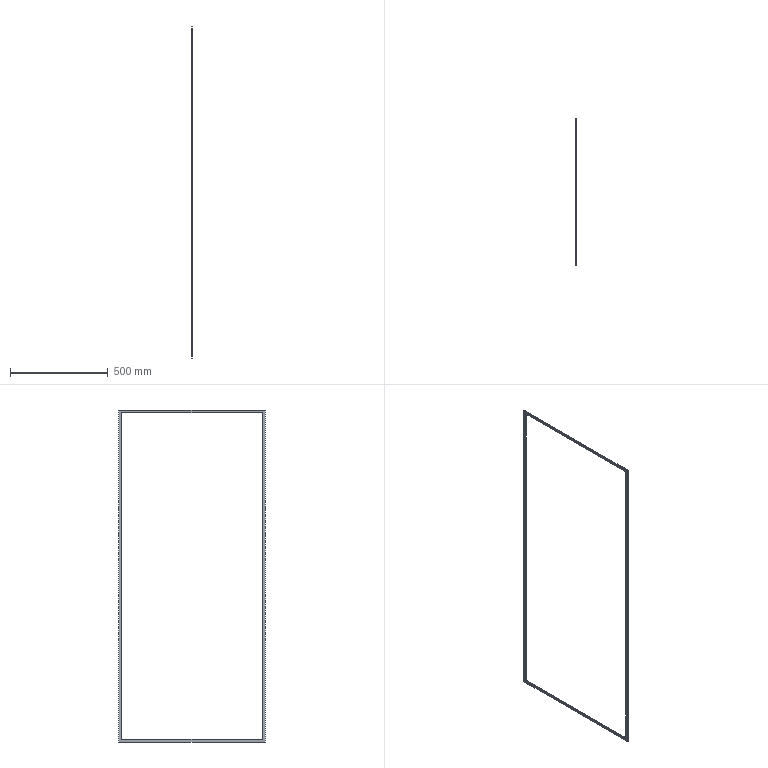Part | STEP file | RJWD-DY-0102_X2_5DE667DC95E8_44 | 1 solid | 10 faces | box 3 x 752 x 1702 mm | volume 218115 mm3 | plane 10
STEP:
#1=CARTESIAN_POINT('',(0.,0.,0.));
#2=DIRECTION('',(0.,0.,1.));
#3=DIRECTION('',(1.,0.,0.));
#4=AXIS2_PLACEMENT_3D('',#1,#2,#3);
#5=CARTESIAN_POINT('',(-521.773,4998.173,1734.894));
#6=VERTEX_POINT('',#5);
#7=CARTESIAN_POINT('',(-521.773,4246.173,1734.894));
#8=VERTEX_POINT('',#7);
#9=CARTESIAN_POINT('',(-521.773,4998.173,1734.894));
#10=DIRECTION('',(0.,-1.,0.));
#11=VECTOR('',#10,1.);
#12=LINE('',#9,#11);
#13=CARTESIAN_POINT('',(-521.773,4622.173,884.144));
#14=DIRECTION('',(-1.,0.,0.));
#15=DIRECTION('',(0.,0.,1.));
#16=AXIS2_PLACEMENT_3D('',#13,#14,#15);
#17=PLANE('',#16);
#18=CARTESIAN_POINT('',(850.75,376.));
#19=DIRECTION('',(0.,-1.));
#20=VECTOR('',#19,1.);
#21=LINE('',#18,#20);
#22=(GEOMETRIC_REPRESENTATION_CONTEXT(2)PARAMETRIC_REPRESENTATION_CONTEXT()REPRESENTATION_CONTEXT('',''));
#23=DEFINITIONAL_REPRESENTATION('',(#21),#22);
#24=PCURVE('',#17,#23);
#25=CARTESIAN_POINT('',(-521.773,4246.173,1734.894));
#26=DIRECTION('',(0.,0.,1.));
#27=DIRECTION('',(0.,-1.,0.));
#28=AXIS2_PLACEMENT_3D('',#25,#26,#27);
#29=PLANE('',#28);
#30=CARTESIAN_POINT('',(-752.,0.));
#31=DIRECTION('',(1.,0.));
#32=VECTOR('',#31,1.);
#33=LINE('',#30,#32);
#34=(GEOMETRIC_REPRESENTATION_CONTEXT(2)PARAMETRIC_REPRESENTATION_CONTEXT()REPRESENTATION_CONTEXT('',''));
#35=DEFINITIONAL_REPRESENTATION('',(#33),#34);
#36=PCURVE('',#29,#35);
#37=SURFACE_CURVE('',#12,(#24,#36),.PCURVE_S1.);
#38=EDGE_CURVE('',#6,#8,#37,.T.);
#39=ORIENTED_EDGE('',*,*,#38,.F.);
#40=CARTESIAN_POINT('',(-521.773,4998.173,33.394));
#41=VERTEX_POINT('',#40);
#42=CARTESIAN_POINT('',(-521.773,4998.173,33.394));
#43=DIRECTION('',(0.,0.,1.));
#44=VECTOR('',#43,1.);
#45=LINE('',#42,#44);
#46=CARTESIAN_POINT('',(-850.75,376.));
#47=DIRECTION('',(1.,0.));
#48=VECTOR('',#47,1.);
#49=LINE('',#46,#48);
#50=(GEOMETRIC_REPRESENTATION_CONTEXT(2)PARAMETRIC_REPRESENTATION_CONTEXT()REPRESENTATION_CONTEXT('',''));
#51=DEFINITIONAL_REPRESENTATION('',(#49),#50);
#52=PCURVE('',#17,#51);
#53=CARTESIAN_POINT('',(-521.773,4998.173,1734.894));
#54=DIRECTION('',(0.,1.,0.));
#55=DIRECTION('',(0.,0.,1.));
#56=AXIS2_PLACEMENT_3D('',#53,#54,#55);
#57=PLANE('',#56);
#58=CARTESIAN_POINT('',(-1701.5,0.));
#59=DIRECTION('',(1.,0.));
#60=VECTOR('',#59,1.);
#61=LINE('',#58,#60);
#62=(GEOMETRIC_REPRESENTATION_CONTEXT(2)PARAMETRIC_REPRESENTATION_CONTEXT()REPRESENTATION_CONTEXT('',''));
#63=DEFINITIONAL_REPRESENTATION('',(#61),#62);
#64=PCURVE('',#57,#63);
#65=SURFACE_CURVE('',#45,(#52,#64),.PCURVE_S1.);
#66=EDGE_CURVE('',#41,#6,#65,.T.);
#67=ORIENTED_EDGE('',*,*,#66,.F.);
#68=CARTESIAN_POINT('',(-521.773,4246.173,33.394));
#69=VERTEX_POINT('',#68);
#70=CARTESIAN_POINT('',(-521.773,4246.173,33.394));
#71=DIRECTION('',(0.,1.,0.));
#72=VECTOR('',#71,1.);
#73=LINE('',#70,#72);
#74=CARTESIAN_POINT('',(-850.75,-376.));
#75=DIRECTION('',(0.,1.));
#76=VECTOR('',#75,1.);
#77=LINE('',#74,#76);
#78=(GEOMETRIC_REPRESENTATION_CONTEXT(2)PARAMETRIC_REPRESENTATION_CONTEXT()REPRESENTATION_CONTEXT('',''));
#79=DEFINITIONAL_REPRESENTATION('',(#77),#78);
#80=PCURVE('',#17,#79);
#81=CARTESIAN_POINT('',(-521.773,4998.173,33.394));
#82=DIRECTION('',(0.,0.,-1.));
#83=DIRECTION('',(0.,1.,0.));
#84=AXIS2_PLACEMENT_3D('',#81,#82,#83);
#85=PLANE('',#84);
#86=CARTESIAN_POINT('',(-752.,0.));
#87=DIRECTION('',(1.,0.));
#88=VECTOR('',#87,1.);
#89=LINE('',#86,#88);
#90=(GEOMETRIC_REPRESENTATION_CONTEXT(2)PARAMETRIC_REPRESENTATION_CONTEXT()REPRESENTATION_CONTEXT('',''));
#91=DEFINITIONAL_REPRESENTATION('',(#89),#90);
#92=PCURVE('',#85,#91);
#93=SURFACE_CURVE('',#73,(#80,#92),.PCURVE_S1.);
#94=EDGE_CURVE('',#69,#41,#93,.T.);
#95=ORIENTED_EDGE('',*,*,#94,.F.);
#96=CARTESIAN_POINT('',(-521.773,4246.173,1734.894));
#97=DIRECTION('',(0.,0.,-1.));
#98=VECTOR('',#97,1.);
#99=LINE('',#96,#98);
#100=CARTESIAN_POINT('',(850.75,-376.));
#101=DIRECTION('',(-1.,0.));
#102=VECTOR('',#101,1.);
#103=LINE('',#100,#102);
#104=(GEOMETRIC_REPRESENTATION_CONTEXT(2)PARAMETRIC_REPRESENTATION_CONTEXT()REPRESENTATION_CONTEXT('',''));
#105=DEFINITIONAL_REPRESENTATION('',(#103),#104);
#106=PCURVE('',#17,#105);
#107=CARTESIAN_POINT('',(-521.773,4246.173,33.394));
#108=DIRECTION('',(0.,-1.,0.));
#109=DIRECTION('',(0.,0.,-1.));
#110=AXIS2_PLACEMENT_3D('',#107,#108,#109);
#111=PLANE('',#110);
#112=CARTESIAN_POINT('',(-1701.5,0.));
#113=DIRECTION('',(1.,0.));
#114=VECTOR('',#113,1.);
#115=LINE('',#112,#114);
#116=(GEOMETRIC_REPRESENTATION_CONTEXT(2)PARAMETRIC_REPRESENTATION_CONTEXT()REPRESENTATION_CONTEXT('',''));
#117=DEFINITIONAL_REPRESENTATION('',(#115),#116);
#118=PCURVE('',#111,#117);
#119=SURFACE_CURVE('',#99,(#106,#118),.PCURVE_S1.);
#120=EDGE_CURVE('',#8,#69,#119,.T.);
#121=ORIENTED_EDGE('',*,*,#120,.F.);
#122=EDGE_LOOP('',(#39,#67,#95,#121));
#123=FACE_BOUND('',#122,.F.);
#124=CARTESIAN_POINT('',(-521.773,4983.173,48.394));
#125=VERTEX_POINT('',#124);
#126=CARTESIAN_POINT('',(-521.773,4261.173,48.394));
#127=VERTEX_POINT('',#126);
#128=CARTESIAN_POINT('',(-521.773,4983.173,48.394));
#129=DIRECTION('',(0.,-1.,0.));
#130=VECTOR('',#129,1.);
#131=LINE('',#128,#130);
#132=CARTESIAN_POINT('',(-835.75,361.));
#133=DIRECTION('',(0.,-1.));
#134=VECTOR('',#133,1.);
#135=LINE('',#132,#134);
#136=(GEOMETRIC_REPRESENTATION_CONTEXT(2)PARAMETRIC_REPRESENTATION_CONTEXT()REPRESENTATION_CONTEXT('',''));
#137=DEFINITIONAL_REPRESENTATION('',(#135),#136);
#138=PCURVE('',#17,#137);
#139=CARTESIAN_POINT('',(-521.773,4261.173,48.394));
#140=DIRECTION('',(0.,0.,1.));
#141=DIRECTION('',(0.,-1.,0.));
#142=AXIS2_PLACEMENT_3D('',#139,#140,#141);
#143=PLANE('',#142);
#144=CARTESIAN_POINT('',(-722.,0.));
#145=DIRECTION('',(1.,0.));
#146=VECTOR('',#145,1.);
#147=LINE('',#144,#146);
#148=(GEOMETRIC_REPRESENTATION_CONTEXT(2)PARAMETRIC_REPRESENTATION_CONTEXT()REPRESENTATION_CONTEXT('',''));
#149=DEFINITIONAL_REPRESENTATION('',(#147),#148);
#150=PCURVE('',#143,#149);
#151=SURFACE_CURVE('',#131,(#138,#150),.PCURVE_S1.);
#152=EDGE_CURVE('',#125,#127,#151,.T.);
#153=ORIENTED_EDGE('',*,*,#152,.F.);
#154=CARTESIAN_POINT('',(-521.773,4983.173,1719.894));
#155=VERTEX_POINT('',#154);
#156=CARTESIAN_POINT('',(-521.773,4983.173,48.394));
#157=DIRECTION('',(0.,0.,1.));
#158=VECTOR('',#157,1.);
#159=LINE('',#156,#158);
#160=CARTESIAN_POINT('',(-835.75,361.));
#161=DIRECTION('',(1.,0.));
#162=VECTOR('',#161,1.);
#163=LINE('',#160,#162);
#164=(GEOMETRIC_REPRESENTATION_CONTEXT(2)PARAMETRIC_REPRESENTATION_CONTEXT()REPRESENTATION_CONTEXT('',''));
#165=DEFINITIONAL_REPRESENTATION('',(#163),#164);
#166=PCURVE('',#17,#165);
#167=CARTESIAN_POINT('',(-521.773,4983.173,48.394));
#168=DIRECTION('',(0.,-1.,0.));
#169=DIRECTION('',(0.,0.,-1.));
#170=AXIS2_PLACEMENT_3D('',#167,#168,#169);
#171=PLANE('',#170);
#172=CARTESIAN_POINT('',(0.,0.));
#173=DIRECTION('',(-1.,0.));
#174=VECTOR('',#173,1.);
#175=LINE('',#172,#174);
#176=(GEOMETRIC_REPRESENTATION_CONTEXT(2)PARAMETRIC_REPRESENTATION_CONTEXT()REPRESENTATION_CONTEXT('',''));
#177=DEFINITIONAL_REPRESENTATION('',(#175),#176);
#178=PCURVE('',#171,#177);
#179=SURFACE_CURVE('',#159,(#166,#178),.PCURVE_S1.);
#180=EDGE_CURVE('',#125,#155,#179,.T.);
#181=ORIENTED_EDGE('',*,*,#180,.T.);
#182=CARTESIAN_POINT('',(-521.773,4261.173,1719.894));
#183=VERTEX_POINT('',#182);
#184=CARTESIAN_POINT('',(-521.773,4261.173,1719.894));
#185=DIRECTION('',(0.,1.,0.));
#186=VECTOR('',#185,1.);
#187=LINE('',#184,#186);
#188=CARTESIAN_POINT('',(835.75,-361.));
#189=DIRECTION('',(0.,1.));
#190=VECTOR('',#189,1.);
#191=LINE('',#188,#190);
#192=(GEOMETRIC_REPRESENTATION_CONTEXT(2)PARAMETRIC_REPRESENTATION_CONTEXT()REPRESENTATION_CONTEXT('',''));
#193=DEFINITIONAL_REPRESENTATION('',(#191),#192);
#194=PCURVE('',#17,#193);
#195=CARTESIAN_POINT('',(-521.773,4983.173,1719.894));
#196=DIRECTION('',(0.,0.,-1.));
#197=DIRECTION('',(0.,1.,0.));
#198=AXIS2_PLACEMENT_3D('',#195,#196,#197);
#199=PLANE('',#198);
#200=CARTESIAN_POINT('',(-722.,0.));
#201=DIRECTION('',(1.,0.));
#202=VECTOR('',#201,1.);
#203=LINE('',#200,#202);
#204=(GEOMETRIC_REPRESENTATION_CONTEXT(2)PARAMETRIC_REPRESENTATION_CONTEXT()REPRESENTATION_CONTEXT('',''));
#205=DEFINITIONAL_REPRESENTATION('',(#203),#204);
#206=PCURVE('',#199,#205);
#207=SURFACE_CURVE('',#187,(#194,#206),.PCURVE_S1.);
#208=EDGE_CURVE('',#183,#155,#207,.T.);
#209=ORIENTED_EDGE('',*,*,#208,.F.);
#210=CARTESIAN_POINT('',(-521.773,4261.173,48.394));
#211=DIRECTION('',(0.,0.,1.));
#212=VECTOR('',#211,1.);
#213=LINE('',#210,#212);
#214=CARTESIAN_POINT('',(-835.75,-361.));
#215=DIRECTION('',(1.,0.));
#216=VECTOR('',#215,1.);
#217=LINE('',#214,#216);
#218=(GEOMETRIC_REPRESENTATION_CONTEXT(2)PARAMETRIC_REPRESENTATION_CONTEXT()REPRESENTATION_CONTEXT('',''));
#219=DEFINITIONAL_REPRESENTATION('',(#217),#218);
#220=PCURVE('',#17,#219);
#221=CARTESIAN_POINT('',(-521.773,4261.173,1719.894));
#222=DIRECTION('',(0.,1.,0.));
#223=DIRECTION('',(0.,0.,1.));
#224=AXIS2_PLACEMENT_3D('',#221,#222,#223);
#225=PLANE('',#224);
#226=CARTESIAN_POINT('',(-1671.5,0.));
#227=DIRECTION('',(1.,0.));
#228=VECTOR('',#227,1.);
#229=LINE('',#226,#228);
#230=(GEOMETRIC_REPRESENTATION_CONTEXT(2)PARAMETRIC_REPRESENTATION_CONTEXT()REPRESENTATION_CONTEXT('',''));
#231=DEFINITIONAL_REPRESENTATION('',(#229),#230);
#232=PCURVE('',#225,#231);
#233=SURFACE_CURVE('',#213,(#220,#232),.PCURVE_S1.);
#234=EDGE_CURVE('',#127,#183,#233,.T.);
#235=ORIENTED_EDGE('',*,*,#234,.F.);
#236=EDGE_LOOP('',(#153,#181,#209,#235));
#237=FACE_BOUND('',#236,.F.);
#238=ADVANCED_FACE('',(#123,#237),#17,.F.);
#239=ORIENTED_EDGE('',*,*,#38,.T.);
#240=CARTESIAN_POINT('',(-524.773,4246.173,1734.894));
#241=VERTEX_POINT('',#240);
#242=CARTESIAN_POINT('',(-524.773,4246.173,1734.894));
#243=DIRECTION('',(1.,0.,0.));
#244=VECTOR('',#243,1.);
#245=LINE('',#242,#244);
#246=CARTESIAN_POINT('',(0.,-3.));
#247=DIRECTION('',(0.,1.));
#248=VECTOR('',#247,1.);
#249=LINE('',#246,#248);
#250=(GEOMETRIC_REPRESENTATION_CONTEXT(2)PARAMETRIC_REPRESENTATION_CONTEXT()REPRESENTATION_CONTEXT('',''));
#251=DEFINITIONAL_REPRESENTATION('',(#249),#250);
#252=PCURVE('',#29,#251);
#253=CARTESIAN_POINT('',(-1701.5,-3.));
#254=DIRECTION('',(0.,1.));
#255=VECTOR('',#254,1.);
#256=LINE('',#253,#255);
#257=(GEOMETRIC_REPRESENTATION_CONTEXT(2)PARAMETRIC_REPRESENTATION_CONTEXT()REPRESENTATION_CONTEXT('',''));
#258=DEFINITIONAL_REPRESENTATION('',(#256),#257);
#259=PCURVE('',#111,#258);
#260=SURFACE_CURVE('',#245,(#252,#259),.PCURVE_S1.);
#261=EDGE_CURVE('',#241,#8,#260,.T.);
#262=ORIENTED_EDGE('',*,*,#261,.F.);
#263=CARTESIAN_POINT('',(-524.773,4998.173,1734.894));
#264=VERTEX_POINT('',#263);
#265=CARTESIAN_POINT('',(-524.773,4998.173,1734.894));
#266=DIRECTION('',(0.,-1.,0.));
#267=VECTOR('',#266,1.);
#268=LINE('',#265,#267);
#269=CARTESIAN_POINT('',(-752.,-3.));
#270=DIRECTION('',(1.,0.));
#271=VECTOR('',#270,1.);
#272=LINE('',#269,#271);
#273=(GEOMETRIC_REPRESENTATION_CONTEXT(2)PARAMETRIC_REPRESENTATION_CONTEXT()REPRESENTATION_CONTEXT('',''));
#274=DEFINITIONAL_REPRESENTATION('',(#272),#273);
#275=PCURVE('',#29,#274);
#276=CARTESIAN_POINT('',(-524.773,4622.173,884.144));
#277=DIRECTION('',(-1.,0.,0.));
#278=DIRECTION('',(0.,0.,1.));
#279=AXIS2_PLACEMENT_3D('',#276,#277,#278);
#280=PLANE('',#279);
#281=CARTESIAN_POINT('',(850.75,376.));
#282=DIRECTION('',(0.,-1.));
#283=VECTOR('',#282,1.);
#284=LINE('',#281,#283);
#285=(GEOMETRIC_REPRESENTATION_CONTEXT(2)PARAMETRIC_REPRESENTATION_CONTEXT()REPRESENTATION_CONTEXT('',''));
#286=DEFINITIONAL_REPRESENTATION('',(#284),#285);
#287=PCURVE('',#280,#286);
#288=SURFACE_CURVE('',#268,(#275,#287),.PCURVE_S1.);
#289=EDGE_CURVE('',#264,#241,#288,.T.);
#290=ORIENTED_EDGE('',*,*,#289,.F.);
#291=CARTESIAN_POINT('',(-524.773,4998.173,1734.894));
#292=DIRECTION('',(1.,0.,0.));
#293=VECTOR('',#292,1.);
#294=LINE('',#291,#293);
#295=CARTESIAN_POINT('',(-752.,-3.));
#296=DIRECTION('',(0.,1.));
#297=VECTOR('',#296,1.);
#298=LINE('',#295,#297);
#299=(GEOMETRIC_REPRESENTATION_CONTEXT(2)PARAMETRIC_REPRESENTATION_CONTEXT()REPRESENTATION_CONTEXT('',''));
#300=DEFINITIONAL_REPRESENTATION('',(#298),#299);
#301=PCURVE('',#29,#300);
#302=CARTESIAN_POINT('',(0.,-3.));
#303=DIRECTION('',(0.,1.));
#304=VECTOR('',#303,1.);
#305=LINE('',#302,#304);
#306=(GEOMETRIC_REPRESENTATION_CONTEXT(2)PARAMETRIC_REPRESENTATION_CONTEXT()REPRESENTATION_CONTEXT('',''));
#307=DEFINITIONAL_REPRESENTATION('',(#305),#306);
#308=PCURVE('',#57,#307);
#309=SURFACE_CURVE('',#294,(#301,#308),.PCURVE_S1.);
#310=EDGE_CURVE('',#264,#6,#309,.T.);
#311=ORIENTED_EDGE('',*,*,#310,.T.);
#312=EDGE_LOOP('',(#239,#262,#290,#311));
#313=FACE_BOUND('',#312,.F.);
#314=ADVANCED_FACE('',(#313),#29,.T.);
#315=ORIENTED_EDGE('',*,*,#261,.T.);
#316=ORIENTED_EDGE('',*,*,#120,.T.);
#317=CARTESIAN_POINT('',(-524.773,4246.173,33.394));
#318=VERTEX_POINT('',#317);
#319=CARTESIAN_POINT('',(-524.773,4246.173,33.394));
#320=DIRECTION('',(1.,0.,0.));
#321=VECTOR('',#320,1.);
#322=LINE('',#319,#321);
#323=CARTESIAN_POINT('',(0.,-3.));
#324=DIRECTION('',(0.,1.));
#325=VECTOR('',#324,1.);
#326=LINE('',#323,#325);
#327=(GEOMETRIC_REPRESENTATION_CONTEXT(2)PARAMETRIC_REPRESENTATION_CONTEXT()REPRESENTATION_CONTEXT('',''));
#328=DEFINITIONAL_REPRESENTATION('',(#326),#327);
#329=PCURVE('',#111,#328);
#330=CARTESIAN_POINT('',(-752.,-3.));
#331=DIRECTION('',(0.,1.));
#332=VECTOR('',#331,1.);
#333=LINE('',#330,#332);
#334=(GEOMETRIC_REPRESENTATION_CONTEXT(2)PARAMETRIC_REPRESENTATION_CONTEXT()REPRESENTATION_CONTEXT('',''));
#335=DEFINITIONAL_REPRESENTATION('',(#333),#334);
#336=PCURVE('',#85,#335);
#337=SURFACE_CURVE('',#322,(#329,#336),.PCURVE_S1.);
#338=EDGE_CURVE('',#318,#69,#337,.T.);
#339=ORIENTED_EDGE('',*,*,#338,.F.);
#340=CARTESIAN_POINT('',(-524.773,4246.173,1734.894));
#341=DIRECTION('',(0.,0.,-1.));
#342=VECTOR('',#341,1.);
#343=LINE('',#340,#342);
#344=CARTESIAN_POINT('',(-1701.5,-3.));
#345=DIRECTION('',(1.,0.));
#346=VECTOR('',#345,1.);
#347=LINE('',#344,#346);
#348=(GEOMETRIC_REPRESENTATION_CONTEXT(2)PARAMETRIC_REPRESENTATION_CONTEXT()REPRESENTATION_CONTEXT('',''));
#349=DEFINITIONAL_REPRESENTATION('',(#347),#348);
#350=PCURVE('',#111,#349);
#351=CARTESIAN_POINT('',(850.75,-376.));
#352=DIRECTION('',(-1.,0.));
#353=VECTOR('',#352,1.);
#354=LINE('',#351,#353);
#355=(GEOMETRIC_REPRESENTATION_CONTEXT(2)PARAMETRIC_REPRESENTATION_CONTEXT()REPRESENTATION_CONTEXT('',''));
#356=DEFINITIONAL_REPRESENTATION('',(#354),#355);
#357=PCURVE('',#280,#356);
#358=SURFACE_CURVE('',#343,(#350,#357),.PCURVE_S1.);
#359=EDGE_CURVE('',#241,#318,#358,.T.);
#360=ORIENTED_EDGE('',*,*,#359,.F.);
#361=EDGE_LOOP('',(#315,#316,#339,#360));
#362=FACE_BOUND('',#361,.F.);
#363=ADVANCED_FACE('',(#362),#111,.T.);
#364=ORIENTED_EDGE('',*,*,#338,.T.);
#365=ORIENTED_EDGE('',*,*,#94,.T.);
#366=CARTESIAN_POINT('',(-524.773,4998.173,33.394));
#367=VERTEX_POINT('',#366);
#368=CARTESIAN_POINT('',(-524.773,4998.173,33.394));
#369=DIRECTION('',(1.,0.,0.));
#370=VECTOR('',#369,1.);
#371=LINE('',#368,#370);
#372=CARTESIAN_POINT('',(0.,-3.));
#373=DIRECTION('',(0.,1.));
#374=VECTOR('',#373,1.);
#375=LINE('',#372,#374);
#376=(GEOMETRIC_REPRESENTATION_CONTEXT(2)PARAMETRIC_REPRESENTATION_CONTEXT()REPRESENTATION_CONTEXT('',''));
#377=DEFINITIONAL_REPRESENTATION('',(#375),#376);
#378=PCURVE('',#85,#377);
#379=CARTESIAN_POINT('',(-1701.5,-3.));
#380=DIRECTION('',(0.,1.));
#381=VECTOR('',#380,1.);
#382=LINE('',#379,#381);
#383=(GEOMETRIC_REPRESENTATION_CONTEXT(2)PARAMETRIC_REPRESENTATION_CONTEXT()REPRESENTATION_CONTEXT('',''));
#384=DEFINITIONAL_REPRESENTATION('',(#382),#383);
#385=PCURVE('',#57,#384);
#386=SURFACE_CURVE('',#371,(#378,#385),.PCURVE_S1.);
#387=EDGE_CURVE('',#367,#41,#386,.T.);
#388=ORIENTED_EDGE('',*,*,#387,.F.);
#389=CARTESIAN_POINT('',(-524.773,4246.173,33.394));
#390=DIRECTION('',(0.,1.,0.));
#391=VECTOR('',#390,1.);
#392=LINE('',#389,#391);
#393=CARTESIAN_POINT('',(-752.,-3.));
#394=DIRECTION('',(1.,0.));
#395=VECTOR('',#394,1.);
#396=LINE('',#393,#395);
#397=(GEOMETRIC_REPRESENTATION_CONTEXT(2)PARAMETRIC_REPRESENTATION_CONTEXT()REPRESENTATION_CONTEXT('',''));
#398=DEFINITIONAL_REPRESENTATION('',(#396),#397);
#399=PCURVE('',#85,#398);
#400=CARTESIAN_POINT('',(-850.75,-376.));
#401=DIRECTION('',(0.,1.));
#402=VECTOR('',#401,1.);
#403=LINE('',#400,#402);
#404=(GEOMETRIC_REPRESENTATION_CONTEXT(2)PARAMETRIC_REPRESENTATION_CONTEXT()REPRESENTATION_CONTEXT('',''));
#405=DEFINITIONAL_REPRESENTATION('',(#403),#404);
#406=PCURVE('',#280,#405);
#407=SURFACE_CURVE('',#392,(#399,#406),.PCURVE_S1.);
#408=EDGE_CURVE('',#318,#367,#407,.T.);
#409=ORIENTED_EDGE('',*,*,#408,.F.);
#410=EDGE_LOOP('',(#364,#365,#388,#409));
#411=FACE_BOUND('',#410,.F.);
#412=ADVANCED_FACE('',(#411),#85,.T.);
#413=ORIENTED_EDGE('',*,*,#387,.T.);
#414=ORIENTED_EDGE('',*,*,#66,.T.);
#415=ORIENTED_EDGE('',*,*,#310,.F.);
#416=CARTESIAN_POINT('',(-524.773,4998.173,33.394));
#417=DIRECTION('',(0.,0.,1.));
#418=VECTOR('',#417,1.);
#419=LINE('',#416,#418);
#420=CARTESIAN_POINT('',(-1701.5,-3.));
#421=DIRECTION('',(1.,0.));
#422=VECTOR('',#421,1.);
#423=LINE('',#420,#422);
#424=(GEOMETRIC_REPRESENTATION_CONTEXT(2)PARAMETRIC_REPRESENTATION_CONTEXT()REPRESENTATION_CONTEXT('',''));
#425=DEFINITIONAL_REPRESENTATION('',(#423),#424);
#426=PCURVE('',#57,#425);
#427=CARTESIAN_POINT('',(-850.75,376.));
#428=DIRECTION('',(1.,0.));
#429=VECTOR('',#428,1.);
#430=LINE('',#427,#429);
#431=(GEOMETRIC_REPRESENTATION_CONTEXT(2)PARAMETRIC_REPRESENTATION_CONTEXT()REPRESENTATION_CONTEXT('',''));
#432=DEFINITIONAL_REPRESENTATION('',(#430),#431);
#433=PCURVE('',#280,#432);
#434=SURFACE_CURVE('',#419,(#426,#433),.PCURVE_S1.);
#435=EDGE_CURVE('',#367,#264,#434,.T.);
#436=ORIENTED_EDGE('',*,*,#435,.F.);
#437=EDGE_LOOP('',(#413,#414,#415,#436));
#438=FACE_BOUND('',#437,.F.);
#439=ADVANCED_FACE('',(#438),#57,.T.);
#440=ORIENTED_EDGE('',*,*,#289,.T.);
#441=ORIENTED_EDGE('',*,*,#359,.T.);
#442=ORIENTED_EDGE('',*,*,#408,.T.);
#443=ORIENTED_EDGE('',*,*,#435,.T.);
#444=EDGE_LOOP('',(#440,#441,#442,#443));
#445=FACE_BOUND('',#444,.F.);
#446=CARTESIAN_POINT('',(-524.773,4983.173,1719.894));
#447=VERTEX_POINT('',#446);
#448=CARTESIAN_POINT('',(-524.773,4983.173,48.394));
#449=VERTEX_POINT('',#448);
#450=CARTESIAN_POINT('',(-524.773,4983.173,1719.894));
#451=DIRECTION('',(0.,0.,-1.));
#452=VECTOR('',#451,1.);
#453=LINE('',#450,#452);
#454=CARTESIAN_POINT('',(835.75,361.));
#455=DIRECTION('',(-1.,0.));
#456=VECTOR('',#455,1.);
#457=LINE('',#454,#456);
#458=(GEOMETRIC_REPRESENTATION_CONTEXT(2)PARAMETRIC_REPRESENTATION_CONTEXT()REPRESENTATION_CONTEXT('',''));
#459=DEFINITIONAL_REPRESENTATION('',(#457),#458);
#460=PCURVE('',#280,#459);
#461=CARTESIAN_POINT('',(-1671.5,-3.));
#462=DIRECTION('',(1.,0.));
#463=VECTOR('',#462,1.);
#464=LINE('',#461,#463);
#465=(GEOMETRIC_REPRESENTATION_CONTEXT(2)PARAMETRIC_REPRESENTATION_CONTEXT()REPRESENTATION_CONTEXT('',''));
#466=DEFINITIONAL_REPRESENTATION('',(#464),#465);
#467=PCURVE('',#171,#466);
#468=SURFACE_CURVE('',#453,(#460,#467),.PCURVE_S1.);
#469=EDGE_CURVE('',#447,#449,#468,.T.);
#470=ORIENTED_EDGE('',*,*,#469,.T.);
#471=CARTESIAN_POINT('',(-524.773,4261.173,48.394));
#472=VERTEX_POINT('',#471);
#473=CARTESIAN_POINT('',(-524.773,4983.173,48.394));
#474=DIRECTION('',(0.,-1.,0.));
#475=VECTOR('',#474,1.);
#476=LINE('',#473,#475);
#477=CARTESIAN_POINT('',(-835.75,361.));
#478=DIRECTION('',(0.,-1.));
#479=VECTOR('',#478,1.);
#480=LINE('',#477,#479);
#481=(GEOMETRIC_REPRESENTATION_CONTEXT(2)PARAMETRIC_REPRESENTATION_CONTEXT()REPRESENTATION_CONTEXT('',''));
#482=DEFINITIONAL_REPRESENTATION('',(#480),#481);
#483=PCURVE('',#280,#482);
#484=CARTESIAN_POINT('',(-722.,-3.));
#485=DIRECTION('',(1.,0.));
#486=VECTOR('',#485,1.);
#487=LINE('',#484,#486);
#488=(GEOMETRIC_REPRESENTATION_CONTEXT(2)PARAMETRIC_REPRESENTATION_CONTEXT()REPRESENTATION_CONTEXT('',''));
#489=DEFINITIONAL_REPRESENTATION('',(#487),#488);
#490=PCURVE('',#143,#489);
#491=SURFACE_CURVE('',#476,(#483,#490),.PCURVE_S1.);
#492=EDGE_CURVE('',#449,#472,#491,.T.);
#493=ORIENTED_EDGE('',*,*,#492,.T.);
#494=CARTESIAN_POINT('',(-524.773,4261.173,1719.894));
#495=VERTEX_POINT('',#494);
#496=CARTESIAN_POINT('',(-524.773,4261.173,48.394));
#497=DIRECTION('',(0.,0.,1.));
#498=VECTOR('',#497,1.);
#499=LINE('',#496,#498);
#500=CARTESIAN_POINT('',(-835.75,-361.));
#501=DIRECTION('',(1.,0.));
#502=VECTOR('',#501,1.);
#503=LINE('',#500,#502);
#504=(GEOMETRIC_REPRESENTATION_CONTEXT(2)PARAMETRIC_REPRESENTATION_CONTEXT()REPRESENTATION_CONTEXT('',''));
#505=DEFINITIONAL_REPRESENTATION('',(#503),#504);
#506=PCURVE('',#280,#505);
#507=CARTESIAN_POINT('',(-1671.5,-3.));
#508=DIRECTION('',(1.,0.));
#509=VECTOR('',#508,1.);
#510=LINE('',#507,#509);
#511=(GEOMETRIC_REPRESENTATION_CONTEXT(2)PARAMETRIC_REPRESENTATION_CONTEXT()REPRESENTATION_CONTEXT('',''));
#512=DEFINITIONAL_REPRESENTATION('',(#510),#511);
#513=PCURVE('',#225,#512);
#514=SURFACE_CURVE('',#499,(#506,#513),.PCURVE_S1.);
#515=EDGE_CURVE('',#472,#495,#514,.T.);
#516=ORIENTED_EDGE('',*,*,#515,.T.);
#517=CARTESIAN_POINT('',(-524.773,4261.173,1719.894));
#518=DIRECTION('',(0.,1.,0.));
#519=VECTOR('',#518,1.);
#520=LINE('',#517,#519);
#521=CARTESIAN_POINT('',(835.75,-361.));
#522=DIRECTION('',(0.,1.));
#523=VECTOR('',#522,1.);
#524=LINE('',#521,#523);
#525=(GEOMETRIC_REPRESENTATION_CONTEXT(2)PARAMETRIC_REPRESENTATION_CONTEXT()REPRESENTATION_CONTEXT('',''));
#526=DEFINITIONAL_REPRESENTATION('',(#524),#525);
#527=PCURVE('',#280,#526);
#528=CARTESIAN_POINT('',(-722.,-3.));
#529=DIRECTION('',(1.,0.));
#530=VECTOR('',#529,1.);
#531=LINE('',#528,#530);
#532=(GEOMETRIC_REPRESENTATION_CONTEXT(2)PARAMETRIC_REPRESENTATION_CONTEXT()REPRESENTATION_CONTEXT('',''));
#533=DEFINITIONAL_REPRESENTATION('',(#531),#532);
#534=PCURVE('',#199,#533);
#535=SURFACE_CURVE('',#520,(#527,#534),.PCURVE_S1.);
#536=EDGE_CURVE('',#495,#447,#535,.T.);
#537=ORIENTED_EDGE('',*,*,#536,.T.);
#538=EDGE_LOOP('',(#470,#493,#516,#537));
#539=FACE_BOUND('',#538,.F.);
#540=ADVANCED_FACE('',(#445,#539),#280,.T.);
#541=ORIENTED_EDGE('',*,*,#180,.F.);
#542=CARTESIAN_POINT('',(-524.773,4983.173,48.394));
#543=DIRECTION('',(1.,0.,0.));
#544=VECTOR('',#543,1.);
#545=LINE('',#542,#544);
#546=CARTESIAN_POINT('',(0.,-3.));
#547=DIRECTION('',(0.,1.));
#548=VECTOR('',#547,1.);
#549=LINE('',#546,#548);
#550=(GEOMETRIC_REPRESENTATION_CONTEXT(2)PARAMETRIC_REPRESENTATION_CONTEXT()REPRESENTATION_CONTEXT('',''));
#551=DEFINITIONAL_REPRESENTATION('',(#549),#550);
#552=PCURVE('',#171,#551);
#553=CARTESIAN_POINT('',(-722.,-3.));
#554=DIRECTION('',(0.,1.));
#555=VECTOR('',#554,1.);
#556=LINE('',#553,#555);
#557=(GEOMETRIC_REPRESENTATION_CONTEXT(2)PARAMETRIC_REPRESENTATION_CONTEXT()REPRESENTATION_CONTEXT('',''));
#558=DEFINITIONAL_REPRESENTATION('',(#556),#557);
#559=PCURVE('',#143,#558);
#560=SURFACE_CURVE('',#545,(#552,#559),.PCURVE_S1.);
#561=EDGE_CURVE('',#449,#125,#560,.T.);
#562=ORIENTED_EDGE('',*,*,#561,.F.);
#563=ORIENTED_EDGE('',*,*,#469,.F.);
#564=CARTESIAN_POINT('',(-524.773,4983.173,1719.894));
#565=DIRECTION('',(1.,0.,0.));
#566=VECTOR('',#565,1.);
#567=LINE('',#564,#566);
#568=CARTESIAN_POINT('',(-1671.5,-3.));
#569=DIRECTION('',(0.,1.));
#570=VECTOR('',#569,1.);
#571=LINE('',#568,#570);
#572=(GEOMETRIC_REPRESENTATION_CONTEXT(2)PARAMETRIC_REPRESENTATION_CONTEXT()REPRESENTATION_CONTEXT('',''));
#573=DEFINITIONAL_REPRESENTATION('',(#571),#572);
#574=PCURVE('',#171,#573);
#575=CARTESIAN_POINT('',(0.,-3.));
#576=DIRECTION('',(0.,1.));
#577=VECTOR('',#576,1.);
#578=LINE('',#575,#577);
#579=(GEOMETRIC_REPRESENTATION_CONTEXT(2)PARAMETRIC_REPRESENTATION_CONTEXT()REPRESENTATION_CONTEXT('',''));
#580=DEFINITIONAL_REPRESENTATION('',(#578),#579);
#581=PCURVE('',#199,#580);
#582=SURFACE_CURVE('',#567,(#574,#581),.PCURVE_S1.);
#583=EDGE_CURVE('',#447,#155,#582,.T.);
#584=ORIENTED_EDGE('',*,*,#583,.T.);
#585=EDGE_LOOP('',(#541,#562,#563,#584));
#586=FACE_BOUND('',#585,.F.);
#587=ADVANCED_FACE('',(#586),#171,.T.);
#588=ORIENTED_EDGE('',*,*,#561,.T.);
#589=ORIENTED_EDGE('',*,*,#152,.T.);
#590=CARTESIAN_POINT('',(-524.773,4261.173,48.394));
#591=DIRECTION('',(1.,0.,0.));
#592=VECTOR('',#591,1.);
#593=LINE('',#590,#592);
#594=CARTESIAN_POINT('',(0.,-3.));
#595=DIRECTION('',(0.,1.));
#596=VECTOR('',#595,1.);
#597=LINE('',#594,#596);
#598=(GEOMETRIC_REPRESENTATION_CONTEXT(2)PARAMETRIC_REPRESENTATION_CONTEXT()REPRESENTATION_CONTEXT('',''));
#599=DEFINITIONAL_REPRESENTATION('',(#597),#598);
#600=PCURVE('',#143,#599);
#601=CARTESIAN_POINT('',(-1671.5,-3.));
#602=DIRECTION('',(0.,1.));
#603=VECTOR('',#602,1.);
#604=LINE('',#601,#603);
#605=(GEOMETRIC_REPRESENTATION_CONTEXT(2)PARAMETRIC_REPRESENTATION_CONTEXT()REPRESENTATION_CONTEXT('',''));
#606=DEFINITIONAL_REPRESENTATION('',(#604),#605);
#607=PCURVE('',#225,#606);
#608=SURFACE_CURVE('',#593,(#600,#607),.PCURVE_S1.);
#609=EDGE_CURVE('',#472,#127,#608,.T.);
#610=ORIENTED_EDGE('',*,*,#609,.F.);
#611=ORIENTED_EDGE('',*,*,#492,.F.);
#612=EDGE_LOOP('',(#588,#589,#610,#611));
#613=FACE_BOUND('',#612,.F.);
#614=ADVANCED_FACE('',(#613),#143,.T.);
#615=ORIENTED_EDGE('',*,*,#609,.T.);
#616=ORIENTED_EDGE('',*,*,#234,.T.);
#617=CARTESIAN_POINT('',(-524.773,4261.173,1719.894));
#618=DIRECTION('',(1.,0.,0.));
#619=VECTOR('',#618,1.);
#620=LINE('',#617,#619);
#621=CARTESIAN_POINT('',(0.,-3.));
#622=DIRECTION('',(0.,1.));
#623=VECTOR('',#622,1.);
#624=LINE('',#621,#623);
#625=(GEOMETRIC_REPRESENTATION_CONTEXT(2)PARAMETRIC_REPRESENTATION_CONTEXT()REPRESENTATION_CONTEXT('',''));
#626=DEFINITIONAL_REPRESENTATION('',(#624),#625);
#627=PCURVE('',#225,#626);
#628=CARTESIAN_POINT('',(-722.,-3.));
#629=DIRECTION('',(0.,1.));
#630=VECTOR('',#629,1.);
#631=LINE('',#628,#630);
#632=(GEOMETRIC_REPRESENTATION_CONTEXT(2)PARAMETRIC_REPRESENTATION_CONTEXT()REPRESENTATION_CONTEXT('',''));
#633=DEFINITIONAL_REPRESENTATION('',(#631),#632);
#634=PCURVE('',#199,#633);
#635=SURFACE_CURVE('',#620,(#627,#634),.PCURVE_S1.);
#636=EDGE_CURVE('',#495,#183,#635,.T.);
#637=ORIENTED_EDGE('',*,*,#636,.F.);
#638=ORIENTED_EDGE('',*,*,#515,.F.);
#639=EDGE_LOOP('',(#615,#616,#637,#638));
#640=FACE_BOUND('',#639,.F.);
#641=ADVANCED_FACE('',(#640),#225,.T.);
#642=ORIENTED_EDGE('',*,*,#208,.T.);
#643=ORIENTED_EDGE('',*,*,#583,.F.);
#644=ORIENTED_EDGE('',*,*,#536,.F.);
#645=ORIENTED_EDGE('',*,*,#636,.T.);
#646=EDGE_LOOP('',(#642,#643,#644,#645));
#647=FACE_BOUND('',#646,.F.);
#648=ADVANCED_FACE('',(#647),#199,.T.);
#649=CLOSED_SHELL('',(#238,#314,#363,#412,#439,#540,#587,#614,#641,#648));
#650=MANIFOLD_SOLID_BREP('',#649);
#651=(LENGTH_UNIT()NAMED_UNIT(*)SI_UNIT(.MILLI.,.METRE.));
#652=UNCERTAINTY_MEASURE_WITH_UNIT(LENGTH_MEASURE(0.0000001),#651,'','');
#653=(NAMED_UNIT(*)PLANE_ANGLE_UNIT()SI_UNIT($,.RADIAN.));
#654=(NAMED_UNIT(*)SI_UNIT($,.STERADIAN.)SOLID_ANGLE_UNIT());
#655=(GEOMETRIC_REPRESENTATION_CONTEXT(3)GLOBAL_UNCERTAINTY_ASSIGNED_CONTEXT((#652))GLOBAL_UNIT_ASSIGNED_CONTEXT((#651,#653,#654))REPRESENTATION_CONTEXT('',''));
#656=ADVANCED_BREP_SHAPE_REPRESENTATION('',(#4,#650),#655);